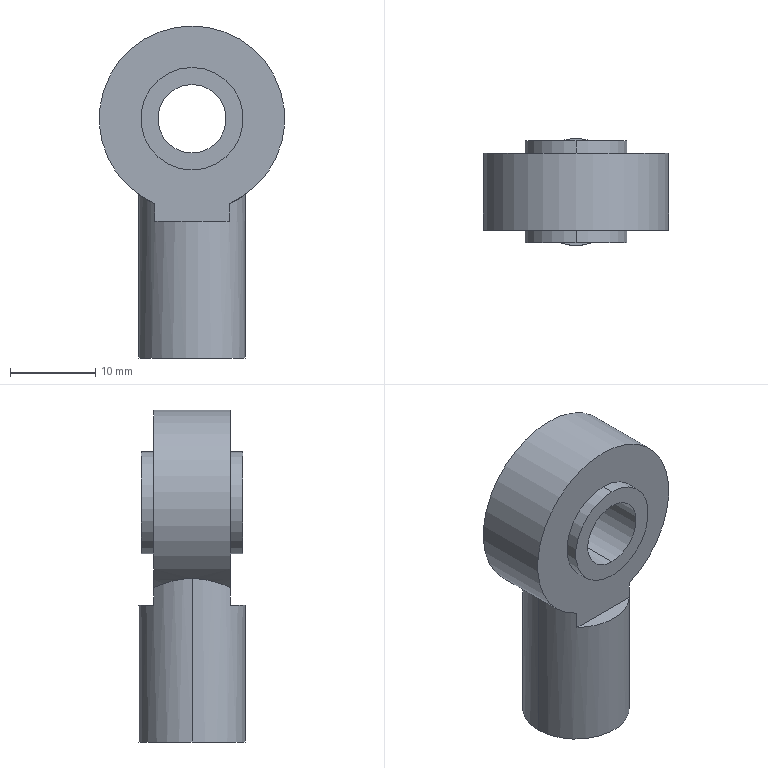Part | SolidWorks | features ICE 4, Extrusion 1, HoleWzd 1 | 1 solid | 20 faces | box 21.7 x 12.5 x 38.85 mm | volume 4732 mm3 | cylinder 11 | plane 7 | cone 2 | commonest cylinder face diameters 12 x4 6.8 x2 8 x2 12.5 x2 21.7 x1
STEP:
#1=CARTESIAN_POINT('',(0.,5.95,24.));
#2=VERTEX_POINT('',#1);
#3=CARTESIAN_POINT('',(0.,5.95,32.));
#4=VERTEX_POINT('',#3);
#5=CARTESIAN_POINT('',(0.,5.95,28.));
#6=DIRECTION('',(0.,1.,0.));
#7=DIRECTION('',(0.,0.,1.));
#8=AXIS2_PLACEMENT_3D('',#5,#6,#7);
#9=CIRCLE('',#8,4.);
#10=EDGE_CURVE('',#2,#4,#9,.T.);
#11=ORIENTED_EDGE('',*,*,#10,.T.);
#12=CARTESIAN_POINT('',(0.,-5.95,32.));
#13=VERTEX_POINT('',#12);
#14=CARTESIAN_POINT('',(0.,6.25,32.));
#15=DIRECTION('',(0.,-1.,0.));
#16=VECTOR('',#15,1000.);
#17=LINE('',#14,#16);
#18=EDGE_CURVE('',#4,#13,#17,.T.);
#19=ORIENTED_EDGE('',*,*,#18,.T.);
#20=CARTESIAN_POINT('',(0.,-5.95,24.));
#21=VERTEX_POINT('',#20);
#22=CARTESIAN_POINT('',(0.,-5.95,28.));
#23=DIRECTION('',(0.,1.,0.));
#24=DIRECTION('',(0.,0.,1.));
#25=AXIS2_PLACEMENT_3D('',#22,#23,#24);
#26=CIRCLE('',#25,4.);
#27=EDGE_CURVE('',#21,#13,#26,.T.);
#28=ORIENTED_EDGE('',*,*,#27,.F.);
#29=CARTESIAN_POINT('',(0.,6.25,24.));
#30=DIRECTION('',(0.,-1.,0.));
#31=VECTOR('',#30,1000.);
#32=LINE('',#29,#31);
#33=EDGE_CURVE('',#2,#21,#32,.T.);
#34=ORIENTED_EDGE('',*,*,#33,.F.);
#35=EDGE_LOOP('',(#11,#19,#28,#34));
#36=FACE_OUTER_BOUND('',#35,.T.);
#37=CARTESIAN_POINT('',(0.,6.25,28.));
#38=DIRECTION('',(0.,-1.,0.));
#39=DIRECTION('',(0.,0.,-1.));
#40=AXIS2_PLACEMENT_3D('',#37,#38,#39);
#41=CYLINDRICAL_SURFACE('',#40,4.);
#42=ADVANCED_FACE('',(#36),#41,.F.);
#43=CARTESIAN_POINT('',(0.,5.95,34.));
#44=VERTEX_POINT('',#43);
#45=CARTESIAN_POINT('',(0.,5.95,22.));
#46=VERTEX_POINT('',#45);
#47=CARTESIAN_POINT('',(0.,5.95,28.));
#48=DIRECTION('',(0.,1.,0.));
#49=DIRECTION('',(0.,0.,1.));
#50=AXIS2_PLACEMENT_3D('',#47,#48,#49);
#51=CIRCLE('',#50,6.);
#52=EDGE_CURVE('',#44,#46,#51,.T.);
#53=ORIENTED_EDGE('',*,*,#52,.F.);
#54=CARTESIAN_POINT('',(0.,4.5,34.));
#55=VERTEX_POINT('',#54);
#56=CARTESIAN_POINT('',(0.,5.95,34.));
#57=DIRECTION('',(0.,-1.,0.));
#58=VECTOR('',#57,1000.);
#59=LINE('',#56,#58);
#60=EDGE_CURVE('',#44,#55,#59,.T.);
#61=ORIENTED_EDGE('',*,*,#60,.T.);
#62=CARTESIAN_POINT('',(0.,4.5,22.));
#63=VERTEX_POINT('',#62);
#64=CARTESIAN_POINT('',(0.,4.5,28.));
#65=DIRECTION('',(0.,-1.,0.));
#66=DIRECTION('',(0.,0.,1.));
#67=AXIS2_PLACEMENT_3D('',#64,#65,#66);
#68=CIRCLE('',#67,6.);
#69=EDGE_CURVE('',#63,#55,#68,.T.);
#70=ORIENTED_EDGE('',*,*,#69,.F.);
#71=CARTESIAN_POINT('',(0.,5.95,22.));
#72=DIRECTION('',(0.,-1.,0.));
#73=VECTOR('',#72,1000.);
#74=LINE('',#71,#73);
#75=EDGE_CURVE('',#46,#63,#74,.T.);
#76=ORIENTED_EDGE('',*,*,#75,.F.);
#77=EDGE_LOOP('',(#53,#61,#70,#76));
#78=FACE_OUTER_BOUND('',#77,.T.);
#79=CARTESIAN_POINT('',(0.,5.95,28.));
#80=DIRECTION('',(0.,-1.,0.));
#81=DIRECTION('',(0.,0.,-1.));
#82=AXIS2_PLACEMENT_3D('',#79,#80,#81);
#83=CYLINDRICAL_SURFACE('',#82,6.);
#84=ADVANCED_FACE('',(#78),#83,.T.);
#85=CARTESIAN_POINT('',(0.,-4.5,22.));
#86=VERTEX_POINT('',#85);
#87=CARTESIAN_POINT('',(0.,-4.5,34.));
#88=VERTEX_POINT('',#87);
#89=CARTESIAN_POINT('',(0.,-4.5,28.));
#90=DIRECTION('',(0.,-1.,0.));
#91=DIRECTION('',(0.,0.,1.));
#92=AXIS2_PLACEMENT_3D('',#89,#90,#91);
#93=CIRCLE('',#92,6.);
#94=EDGE_CURVE('',#86,#88,#93,.T.);
#95=ORIENTED_EDGE('',*,*,#94,.T.);
#96=CARTESIAN_POINT('',(0.,-5.95,34.));
#97=VERTEX_POINT('',#96);
#98=CARTESIAN_POINT('',(0.,5.95,34.));
#99=DIRECTION('',(0.,-1.,0.));
#100=VECTOR('',#99,1000.);
#101=LINE('',#98,#100);
#102=EDGE_CURVE('',#88,#97,#101,.T.);
#103=ORIENTED_EDGE('',*,*,#102,.T.);
#104=CARTESIAN_POINT('',(0.,-5.95,22.));
#105=VERTEX_POINT('',#104);
#106=CARTESIAN_POINT('',(0.,-5.95,28.));
#107=DIRECTION('',(0.,1.,0.));
#108=DIRECTION('',(0.,0.,1.));
#109=AXIS2_PLACEMENT_3D('',#106,#107,#108);
#110=CIRCLE('',#109,6.);
#111=EDGE_CURVE('',#97,#105,#110,.T.);
#112=ORIENTED_EDGE('',*,*,#111,.T.);
#113=CARTESIAN_POINT('',(0.,5.95,22.));
#114=DIRECTION('',(0.,-1.,0.));
#115=VECTOR('',#114,1000.);
#116=LINE('',#113,#115);
#117=EDGE_CURVE('',#86,#105,#116,.T.);
#118=ORIENTED_EDGE('',*,*,#117,.F.);
#119=EDGE_LOOP('',(#95,#103,#112,#118));
#120=FACE_OUTER_BOUND('',#119,.T.);
#121=CARTESIAN_POINT('',(0.,5.95,28.));
#122=DIRECTION('',(0.,-1.,0.));
#123=DIRECTION('',(0.,0.,-1.));
#124=AXIS2_PLACEMENT_3D('',#121,#122,#123);
#125=CYLINDRICAL_SURFACE('',#124,6.);
#126=ADVANCED_FACE('',(#120),#125,.T.);
#127=CARTESIAN_POINT('',(3.4,0.,12.));
#128=VERTEX_POINT('',#127);
#129=CARTESIAN_POINT('',(-3.4,0.,12.));
#130=VERTEX_POINT('',#129);
#131=CARTESIAN_POINT('',(0.,0.,12.));
#132=DIRECTION('',(0.,0.,-1.));
#133=DIRECTION('',(-1.,0.,0.));
#134=AXIS2_PLACEMENT_3D('',#131,#132,#133);
#135=CIRCLE('',#134,3.4);
#136=EDGE_CURVE('',#128,#130,#135,.T.);
#137=ORIENTED_EDGE('',*,*,#136,.F.);
#138=CARTESIAN_POINT('',(3.4,0.,0.));
#139=VERTEX_POINT('',#138);
#140=CARTESIAN_POINT('',(3.4,0.,0.));
#141=DIRECTION('',(0.,0.,-1.));
#142=VECTOR('',#141,1000.);
#143=LINE('',#140,#142);
#144=EDGE_CURVE('',#128,#139,#143,.T.);
#145=ORIENTED_EDGE('',*,*,#144,.T.);
#146=CARTESIAN_POINT('',(-3.4,0.,0.));
#147=VERTEX_POINT('',#146);
#148=CARTESIAN_POINT('',(0.,0.,0.));
#149=DIRECTION('',(0.,0.,-1.));
#150=DIRECTION('',(-1.,0.,0.));
#151=AXIS2_PLACEMENT_3D('',#148,#149,#150);
#152=CIRCLE('',#151,3.4);
#153=EDGE_CURVE('',#139,#147,#152,.T.);
#154=ORIENTED_EDGE('',*,*,#153,.T.);
#155=CARTESIAN_POINT('',(-3.4,0.,0.));
#156=DIRECTION('',(0.,0.,-1.));
#157=VECTOR('',#156,1000.);
#158=LINE('',#155,#157);
#159=EDGE_CURVE('',#130,#147,#158,.T.);
#160=ORIENTED_EDGE('',*,*,#159,.F.);
#161=EDGE_LOOP('',(#137,#145,#154,#160));
#162=FACE_OUTER_BOUND('',#161,.T.);
#163=CARTESIAN_POINT('',(0.,0.,0.));
#164=DIRECTION('',(0.,0.,-1.));
#165=DIRECTION('',(-1.,0.,0.));
#166=AXIS2_PLACEMENT_3D('',#163,#164,#165);
#167=CYLINDRICAL_SURFACE('',#166,3.4);
#168=ADVANCED_FACE('',(#162),#167,.F.);
#169=CARTESIAN_POINT('',(0.,0.,14.043));
#170=VERTEX_POINT('',#169);
#171=CARTESIAN_POINT('',(-3.4,0.,12.));
#172=DIRECTION('',(-0.8572,0.,-0.515));
#173=VECTOR('',#172,1000.);
#174=LINE('',#171,#173);
#175=EDGE_CURVE('',#170,#130,#174,.T.);
#176=ORIENTED_EDGE('',*,*,#175,.F.);
#177=CARTESIAN_POINT('',(3.4,0.,12.));
#178=DIRECTION('',(0.8572,0.,-0.515));
#179=VECTOR('',#178,1000.);
#180=LINE('',#177,#179);
#181=EDGE_CURVE('',#170,#128,#180,.T.);
#182=ORIENTED_EDGE('',*,*,#181,.T.);
#183=ORIENTED_EDGE('',*,*,#136,.T.);
#184=EDGE_LOOP('',(#176,#182,#183));
#185=FACE_OUTER_BOUND('',#184,.T.);
#186=CARTESIAN_POINT('',(0.,0.,12.));
#187=DIRECTION('',(0.,0.,-1.));
#188=DIRECTION('',(-1.,0.,0.));
#189=AXIS2_PLACEMENT_3D('',#186,#187,#188);
#190=CONICAL_SURFACE('',#189,3.4,1.03);
#191=ADVANCED_FACE('',(#185),#190,.F.);
#192=CARTESIAN_POINT('',(6.25,0.,19.131));
#193=VERTEX_POINT('',#192);
#194=CARTESIAN_POINT('',(4.337,4.5,18.055));
#195=VERTEX_POINT('',#194);
#196=CARTESIAN_POINT('',(6.25,0.,19.131));
#197=CARTESIAN_POINT('',(6.25,0.4269,19.131));
#198=CARTESIAN_POINT('',(6.206,0.8535,19.1));
#199=CARTESIAN_POINT('',(6.032,1.693,18.98));
#200=CARTESIAN_POINT('',(5.904,2.094,18.895));
#201=CARTESIAN_POINT('',(5.655,2.669,18.74));
#202=CARTESIAN_POINT('',(5.562,2.857,18.684));
#203=CARTESIAN_POINT('',(5.361,3.22,18.566));
#204=CARTESIAN_POINT('',(5.252,3.394,18.505));
#205=CARTESIAN_POINT('',(4.901,3.9,18.317));
#206=CARTESIAN_POINT('',(4.635,4.213,18.184));
#207=CARTESIAN_POINT('',(4.337,4.5,18.055));
#208=B_SPLINE_CURVE_WITH_KNOTS('',3,(#196,#197,#198,#199,#200,#201,#202,#203,#204,#205,#206,#207),.UNSPECIFIED.,.F.,.F.,(4,2,2,2,2,4),(0.005141,0.006422,0.007703,0.008344,0.008985,0.01027),.UNSPECIFIED.);
#209=EDGE_CURVE('',#193,#195,#208,.T.);
#210=ORIENTED_EDGE('',*,*,#209,.F.);
#211=CARTESIAN_POINT('',(6.25,0.,0.));
#212=VERTEX_POINT('',#211);
#213=CARTESIAN_POINT('',(6.25,0.,28.));
#214=DIRECTION('',(0.,0.,-1.));
#215=VECTOR('',#214,1000.);
#216=LINE('',#213,#215);
#217=EDGE_CURVE('',#193,#212,#216,.T.);
#218=ORIENTED_EDGE('',*,*,#217,.T.);
#219=CARTESIAN_POINT('',(-6.25,0.,0.));
#220=VERTEX_POINT('',#219);
#221=CARTESIAN_POINT('',(0.,0.,0.));
#222=DIRECTION('',(0.,0.,1.));
#223=DIRECTION('',(1.,0.,0.));
#224=AXIS2_PLACEMENT_3D('',#221,#222,#223);
#225=CIRCLE('',#224,6.25);
#226=EDGE_CURVE('',#212,#220,#225,.T.);
#227=ORIENTED_EDGE('',*,*,#226,.T.);
#228=CARTESIAN_POINT('',(-6.25,0.,19.131));
#229=VERTEX_POINT('',#228);
#230=CARTESIAN_POINT('',(-6.25,0.,28.));
#231=DIRECTION('',(0.,0.,-1.));
#232=VECTOR('',#231,1000.);
#233=LINE('',#230,#232);
#234=EDGE_CURVE('',#229,#220,#233,.T.);
#235=ORIENTED_EDGE('',*,*,#234,.F.);
#236=CARTESIAN_POINT('',(-4.337,4.5,18.055));
#237=VERTEX_POINT('',#236);
#238=CARTESIAN_POINT('',(-4.337,4.5,18.055));
#239=CARTESIAN_POINT('',(-4.635,4.213,18.185));
#240=CARTESIAN_POINT('',(-4.9,3.901,18.316));
#241=CARTESIAN_POINT('',(-5.251,3.396,18.504));
#242=CARTESIAN_POINT('',(-5.36,3.222,18.566));
#243=CARTESIAN_POINT('',(-5.562,2.859,18.683));
#244=CARTESIAN_POINT('',(-5.655,2.67,18.74));
#245=CARTESIAN_POINT('',(-5.903,2.095,18.894));
#246=CARTESIAN_POINT('',(-6.03,1.696,18.98));
#247=CARTESIAN_POINT('',(-6.161,1.073,19.069));
#248=CARTESIAN_POINT('',(-6.194,0.8594,19.092));
#249=CARTESIAN_POINT('',(-6.239,0.4288,19.123));
#250=CARTESIAN_POINT('',(-6.25,0.2141,19.131));
#251=CARTESIAN_POINT('',(-6.25,0.,19.131));
#252=B_SPLINE_CURVE_WITH_KNOTS('',3,(#238,#239,#240,#241,#242,#243,#244,#245,#246,#247,#248,#249,#250,#251),.UNSPECIFIED.,.F.,.F.,(4,2,2,2,2,2,4),(0.,0.001285,0.001928,0.00257,0.003856,0.004498,0.005141),.UNSPECIFIED.);
#253=EDGE_CURVE('',#237,#229,#252,.T.);
#254=ORIENTED_EDGE('',*,*,#253,.F.);
#255=CARTESIAN_POINT('',(-4.337,4.5,16.));
#256=VERTEX_POINT('',#255);
#257=CARTESIAN_POINT('',(-4.337,4.5,16.));
#258=DIRECTION('',(0.,0.,1.));
#259=VECTOR('',#258,1000.);
#260=LINE('',#257,#259);
#261=EDGE_CURVE('',#256,#237,#260,.T.);
#262=ORIENTED_EDGE('',*,*,#261,.F.);
#263=CARTESIAN_POINT('',(4.337,4.5,16.));
#264=VERTEX_POINT('',#263);
#265=CARTESIAN_POINT('',(0.,0.,16.));
#266=DIRECTION('',(0.,0.,1.));
#267=DIRECTION('',(1.,0.,0.));
#268=AXIS2_PLACEMENT_3D('',#265,#266,#267);
#269=CIRCLE('',#268,6.25);
#270=EDGE_CURVE('',#264,#256,#269,.T.);
#271=ORIENTED_EDGE('',*,*,#270,.F.);
#272=CARTESIAN_POINT('',(4.337,4.5,16.));
#273=DIRECTION('',(0.,0.,1.));
#274=VECTOR('',#273,1000.);
#275=LINE('',#272,#274);
#276=EDGE_CURVE('',#264,#195,#275,.T.);
#277=ORIENTED_EDGE('',*,*,#276,.T.);
#278=EDGE_LOOP('',(#210,#218,#227,#235,#254,#262,#271,#277));
#279=FACE_OUTER_BOUND('',#278,.T.);
#280=CARTESIAN_POINT('',(0.,0.,28.));
#281=DIRECTION('',(0.,0.,-1.));
#282=DIRECTION('',(-1.,0.,0.));
#283=AXIS2_PLACEMENT_3D('',#280,#281,#282);
#284=CYLINDRICAL_SURFACE('',#283,6.25);
#285=ADVANCED_FACE('',(#279),#284,.T.);
#286=CARTESIAN_POINT('',(0.,4.5,28.));
#287=DIRECTION('',(0.,1.,0.));
#288=DIRECTION('',(0.,0.,1.));
#289=AXIS2_PLACEMENT_3D('',#286,#287,#288);
#290=CIRCLE('',#289,10.85);
#291=EDGE_CURVE('',#237,#195,#290,.T.);
#292=ORIENTED_EDGE('',*,*,#291,.T.);
#293=ORIENTED_EDGE('',*,*,#276,.F.);
#294=CARTESIAN_POINT('',(-4.337,4.5,16.));
#295=DIRECTION('',(1.,0.,0.));
#296=VECTOR('',#295,1000.);
#297=LINE('',#294,#296);
#298=EDGE_CURVE('',#256,#264,#297,.T.);
#299=ORIENTED_EDGE('',*,*,#298,.F.);
#300=ORIENTED_EDGE('',*,*,#261,.T.);
#301=EDGE_LOOP('',(#292,#293,#299,#300));
#302=FACE_OUTER_BOUND('',#301,.T.);
#303=ORIENTED_EDGE('',*,*,#69,.T.);
#304=CARTESIAN_POINT('',(0.,4.5,28.));
#305=DIRECTION('',(0.,-1.,0.));
#306=DIRECTION('',(0.,0.,1.));
#307=AXIS2_PLACEMENT_3D('',#304,#305,#306);
#308=CIRCLE('',#307,6.);
#309=EDGE_CURVE('',#55,#63,#308,.T.);
#310=ORIENTED_EDGE('',*,*,#309,.T.);
#311=EDGE_LOOP('',(#303,#310));
#312=FACE_BOUND('',#311,.T.);
#313=CARTESIAN_POINT('',(0.,4.5,28.));
#314=DIRECTION('',(0.,1.,0.));
#315=DIRECTION('',(0.,0.,1.));
#316=AXIS2_PLACEMENT_3D('',#313,#314,#315);
#317=PLANE('',#316);
#318=ADVANCED_FACE('',(#302,#312),#317,.T.);
#319=CARTESIAN_POINT('',(4.337,-4.5,16.));
#320=VERTEX_POINT('',#319);
#321=CARTESIAN_POINT('',(4.337,-4.5,18.055));
#322=VERTEX_POINT('',#321);
#323=CARTESIAN_POINT('',(4.337,-4.5,16.));
#324=DIRECTION('',(0.,0.,1.));
#325=VECTOR('',#324,1000.);
#326=LINE('',#323,#325);
#327=EDGE_CURVE('',#320,#322,#326,.T.);
#328=ORIENTED_EDGE('',*,*,#327,.T.);
#329=CARTESIAN_POINT('',(-4.337,-4.5,18.055));
#330=VERTEX_POINT('',#329);
#331=CARTESIAN_POINT('',(0.,-4.5,28.));
#332=DIRECTION('',(0.,1.,0.));
#333=DIRECTION('',(0.,0.,1.));
#334=AXIS2_PLACEMENT_3D('',#331,#332,#333);
#335=CIRCLE('',#334,10.85);
#336=EDGE_CURVE('',#330,#322,#335,.T.);
#337=ORIENTED_EDGE('',*,*,#336,.F.);
#338=CARTESIAN_POINT('',(-4.337,-4.5,16.));
#339=VERTEX_POINT('',#338);
#340=CARTESIAN_POINT('',(-4.337,-4.5,16.));
#341=DIRECTION('',(0.,0.,1.));
#342=VECTOR('',#341,1000.);
#343=LINE('',#340,#342);
#344=EDGE_CURVE('',#339,#330,#343,.T.);
#345=ORIENTED_EDGE('',*,*,#344,.F.);
#346=CARTESIAN_POINT('',(4.337,-4.5,16.));
#347=DIRECTION('',(-1.,0.,0.));
#348=VECTOR('',#347,1000.);
#349=LINE('',#346,#348);
#350=EDGE_CURVE('',#320,#339,#349,.T.);
#351=ORIENTED_EDGE('',*,*,#350,.F.);
#352=EDGE_LOOP('',(#328,#337,#345,#351));
#353=FACE_OUTER_BOUND('',#352,.T.);
#354=ORIENTED_EDGE('',*,*,#94,.F.);
#355=CARTESIAN_POINT('',(0.,-4.5,28.));
#356=DIRECTION('',(0.,-1.,0.));
#357=DIRECTION('',(0.,0.,1.));
#358=AXIS2_PLACEMENT_3D('',#355,#356,#357);
#359=CIRCLE('',#358,6.);
#360=EDGE_CURVE('',#88,#86,#359,.T.);
#361=ORIENTED_EDGE('',*,*,#360,.F.);
#362=EDGE_LOOP('',(#354,#361));
#363=FACE_BOUND('',#362,.T.);
#364=CARTESIAN_POINT('',(0.,-4.5,28.));
#365=DIRECTION('',(0.,1.,0.));
#366=DIRECTION('',(0.,0.,1.));
#367=AXIS2_PLACEMENT_3D('',#364,#365,#366);
#368=PLANE('',#367);
#369=ADVANCED_FACE('',(#353,#363),#368,.F.);
#370=ORIENTED_EDGE('',*,*,#217,.F.);
#371=CARTESIAN_POINT('',(4.337,-4.5,18.055));
#372=CARTESIAN_POINT('',(4.635,-4.213,18.185));
#373=CARTESIAN_POINT('',(4.9,-3.901,18.316));
#374=CARTESIAN_POINT('',(5.251,-3.396,18.504));
#375=CARTESIAN_POINT('',(5.36,-3.222,18.566));
#376=CARTESIAN_POINT('',(5.562,-2.859,18.683));
#377=CARTESIAN_POINT('',(5.655,-2.67,18.74));
#378=CARTESIAN_POINT('',(5.903,-2.095,18.894));
#379=CARTESIAN_POINT('',(6.03,-1.696,18.98));
#380=CARTESIAN_POINT('',(6.161,-1.073,19.069));
#381=CARTESIAN_POINT('',(6.194,-0.8594,19.092));
#382=CARTESIAN_POINT('',(6.239,-0.4288,19.123));
#383=CARTESIAN_POINT('',(6.25,-0.2141,19.131));
#384=CARTESIAN_POINT('',(6.25,0.,19.131));
#385=B_SPLINE_CURVE_WITH_KNOTS('',3,(#371,#372,#373,#374,#375,#376,#377,#378,#379,#380,#381,#382,#383,#384),.UNSPECIFIED.,.F.,.F.,(4,2,2,2,2,2,4),(0.,0.001285,0.001928,0.00257,0.003856,0.004498,0.005141),.UNSPECIFIED.);
#386=EDGE_CURVE('',#322,#193,#385,.T.);
#387=ORIENTED_EDGE('',*,*,#386,.F.);
#388=ORIENTED_EDGE('',*,*,#327,.F.);
#389=CARTESIAN_POINT('',(0.,0.,16.));
#390=DIRECTION('',(0.,0.,1.));
#391=DIRECTION('',(1.,0.,0.));
#392=AXIS2_PLACEMENT_3D('',#389,#390,#391);
#393=CIRCLE('',#392,6.25);
#394=EDGE_CURVE('',#339,#320,#393,.T.);
#395=ORIENTED_EDGE('',*,*,#394,.F.);
#396=ORIENTED_EDGE('',*,*,#344,.T.);
#397=CARTESIAN_POINT('',(-6.25,0.,19.131));
#398=CARTESIAN_POINT('',(-6.25,-0.4269,19.131));
#399=CARTESIAN_POINT('',(-6.206,-0.8535,19.1));
#400=CARTESIAN_POINT('',(-6.032,-1.693,18.98));
#401=CARTESIAN_POINT('',(-5.904,-2.094,18.895));
#402=CARTESIAN_POINT('',(-5.655,-2.669,18.74));
#403=CARTESIAN_POINT('',(-5.562,-2.857,18.684));
#404=CARTESIAN_POINT('',(-5.361,-3.22,18.566));
#405=CARTESIAN_POINT('',(-5.252,-3.394,18.505));
#406=CARTESIAN_POINT('',(-4.901,-3.9,18.317));
#407=CARTESIAN_POINT('',(-4.635,-4.213,18.184));
#408=CARTESIAN_POINT('',(-4.337,-4.5,18.055));
#409=B_SPLINE_CURVE_WITH_KNOTS('',3,(#397,#398,#399,#400,#401,#402,#403,#404,#405,#406,#407,#408),.UNSPECIFIED.,.F.,.F.,(4,2,2,2,2,4),(0.005141,0.006422,0.007703,0.008344,0.008985,0.01027),.UNSPECIFIED.);
#410=EDGE_CURVE('',#229,#330,#409,.T.);
#411=ORIENTED_EDGE('',*,*,#410,.F.);
#412=ORIENTED_EDGE('',*,*,#234,.T.);
#413=CARTESIAN_POINT('',(0.,0.,0.));
#414=DIRECTION('',(0.,0.,1.));
#415=DIRECTION('',(1.,0.,0.));
#416=AXIS2_PLACEMENT_3D('',#413,#414,#415);
#417=CIRCLE('',#416,6.25);
#418=EDGE_CURVE('',#220,#212,#417,.T.);
#419=ORIENTED_EDGE('',*,*,#418,.T.);
#420=EDGE_LOOP('',(#370,#387,#388,#395,#396,#411,#412,#419));
#421=FACE_OUTER_BOUND('',#420,.T.);
#422=CARTESIAN_POINT('',(0.,0.,28.));
#423=DIRECTION('',(0.,0.,-1.));
#424=DIRECTION('',(-1.,0.,0.));
#425=AXIS2_PLACEMENT_3D('',#422,#423,#424);
#426=CYLINDRICAL_SURFACE('',#425,6.25);
#427=ADVANCED_FACE('',(#421),#426,.T.);
#428=CARTESIAN_POINT('',(0.,0.,0.));
#429=DIRECTION('',(0.,0.,-1.));
#430=DIRECTION('',(-1.,0.,0.));
#431=AXIS2_PLACEMENT_3D('',#428,#429,#430);
#432=CIRCLE('',#431,3.4);
#433=EDGE_CURVE('',#147,#139,#432,.T.);
#434=ORIENTED_EDGE('',*,*,#433,.F.);
#435=ORIENTED_EDGE('',*,*,#153,.F.);
#436=EDGE_LOOP('',(#434,#435));
#437=FACE_BOUND('',#436,.T.);
#438=ORIENTED_EDGE('',*,*,#418,.F.);
#439=ORIENTED_EDGE('',*,*,#226,.F.);
#440=EDGE_LOOP('',(#438,#439));
#441=FACE_OUTER_BOUND('',#440,.T.);
#442=CARTESIAN_POINT('',(0.,0.,0.));
#443=DIRECTION('',(0.,0.,1.));
#444=DIRECTION('',(1.,0.,0.));
#445=AXIS2_PLACEMENT_3D('',#442,#443,#444);
#446=PLANE('',#445);
#447=ADVANCED_FACE('',(#437,#441),#446,.F.);
#448=ORIENTED_EDGE('',*,*,#291,.F.);
#449=ORIENTED_EDGE('',*,*,#253,.T.);
#450=ORIENTED_EDGE('',*,*,#410,.T.);
#451=ORIENTED_EDGE('',*,*,#336,.T.);
#452=ORIENTED_EDGE('',*,*,#386,.T.);
#453=ORIENTED_EDGE('',*,*,#209,.T.);
#454=EDGE_LOOP('',(#448,#449,#450,#451,#452,#453));
#455=FACE_OUTER_BOUND('',#454,.T.);
#456=CARTESIAN_POINT('',(0.,4.5,28.));
#457=DIRECTION('',(0.,-1.,0.));
#458=DIRECTION('',(0.,0.,-1.));
#459=AXIS2_PLACEMENT_3D('',#456,#457,#458);
#460=CYLINDRICAL_SURFACE('',#459,10.85);
#461=ADVANCED_FACE('',(#455),#460,.T.);
#462=ORIENTED_EDGE('',*,*,#270,.T.);
#463=ORIENTED_EDGE('',*,*,#298,.T.);
#464=EDGE_LOOP('',(#462,#463));
#465=FACE_OUTER_BOUND('',#464,.T.);
#466=CARTESIAN_POINT('',(0.,0.,16.));
#467=DIRECTION('',(0.,0.,1.));
#468=DIRECTION('',(1.,0.,0.));
#469=AXIS2_PLACEMENT_3D('',#466,#467,#468);
#470=PLANE('',#469);
#471=ADVANCED_FACE('',(#465),#470,.T.);
#472=ORIENTED_EDGE('',*,*,#394,.T.);
#473=ORIENTED_EDGE('',*,*,#350,.T.);
#474=EDGE_LOOP('',(#472,#473));
#475=FACE_OUTER_BOUND('',#474,.T.);
#476=CARTESIAN_POINT('',(0.,0.,16.));
#477=DIRECTION('',(0.,0.,1.));
#478=DIRECTION('',(1.,0.,0.));
#479=AXIS2_PLACEMENT_3D('',#476,#477,#478);
#480=PLANE('',#479);
#481=ADVANCED_FACE('',(#475),#480,.T.);
#482=ORIENTED_EDGE('',*,*,#181,.F.);
#483=ORIENTED_EDGE('',*,*,#175,.T.);
#484=CARTESIAN_POINT('',(0.,0.,12.));
#485=DIRECTION('',(0.,0.,-1.));
#486=DIRECTION('',(-1.,0.,0.));
#487=AXIS2_PLACEMENT_3D('',#484,#485,#486);
#488=CIRCLE('',#487,3.4);
#489=EDGE_CURVE('',#130,#128,#488,.T.);
#490=ORIENTED_EDGE('',*,*,#489,.T.);
#491=EDGE_LOOP('',(#482,#483,#490));
#492=FACE_OUTER_BOUND('',#491,.T.);
#493=CARTESIAN_POINT('',(0.,0.,12.));
#494=DIRECTION('',(0.,0.,-1.));
#495=DIRECTION('',(-1.,0.,0.));
#496=AXIS2_PLACEMENT_3D('',#493,#494,#495);
#497=CONICAL_SURFACE('',#496,3.4,1.03);
#498=ADVANCED_FACE('',(#492),#497,.F.);
#499=ORIENTED_EDGE('',*,*,#144,.F.);
#500=ORIENTED_EDGE('',*,*,#489,.F.);
#501=ORIENTED_EDGE('',*,*,#159,.T.);
#502=ORIENTED_EDGE('',*,*,#433,.T.);
#503=EDGE_LOOP('',(#499,#500,#501,#502));
#504=FACE_OUTER_BOUND('',#503,.T.);
#505=CARTESIAN_POINT('',(0.,0.,0.));
#506=DIRECTION('',(0.,0.,-1.));
#507=DIRECTION('',(-1.,0.,0.));
#508=AXIS2_PLACEMENT_3D('',#505,#506,#507);
#509=CYLINDRICAL_SURFACE('',#508,3.4);
#510=ADVANCED_FACE('',(#504),#509,.F.);
#511=ORIENTED_EDGE('',*,*,#102,.F.);
#512=ORIENTED_EDGE('',*,*,#360,.T.);
#513=ORIENTED_EDGE('',*,*,#117,.T.);
#514=CARTESIAN_POINT('',(0.,-5.95,28.));
#515=DIRECTION('',(0.,1.,0.));
#516=DIRECTION('',(0.,0.,1.));
#517=AXIS2_PLACEMENT_3D('',#514,#515,#516);
#518=CIRCLE('',#517,6.);
#519=EDGE_CURVE('',#105,#97,#518,.T.);
#520=ORIENTED_EDGE('',*,*,#519,.T.);
#521=EDGE_LOOP('',(#511,#512,#513,#520));
#522=FACE_OUTER_BOUND('',#521,.T.);
#523=CARTESIAN_POINT('',(0.,5.95,28.));
#524=DIRECTION('',(0.,-1.,0.));
#525=DIRECTION('',(0.,0.,-1.));
#526=AXIS2_PLACEMENT_3D('',#523,#524,#525);
#527=CYLINDRICAL_SURFACE('',#526,6.);
#528=ADVANCED_FACE('',(#522),#527,.T.);
#529=ORIENTED_EDGE('',*,*,#519,.F.);
#530=ORIENTED_EDGE('',*,*,#111,.F.);
#531=EDGE_LOOP('',(#529,#530));
#532=FACE_OUTER_BOUND('',#531,.T.);
#533=ORIENTED_EDGE('',*,*,#27,.T.);
#534=CARTESIAN_POINT('',(0.,-5.95,28.));
#535=DIRECTION('',(0.,1.,0.));
#536=DIRECTION('',(0.,0.,1.));
#537=AXIS2_PLACEMENT_3D('',#534,#535,#536);
#538=CIRCLE('',#537,4.);
#539=EDGE_CURVE('',#13,#21,#538,.T.);
#540=ORIENTED_EDGE('',*,*,#539,.T.);
#541=EDGE_LOOP('',(#533,#540));
#542=FACE_BOUND('',#541,.T.);
#543=CARTESIAN_POINT('',(0.,-5.95,28.));
#544=DIRECTION('',(0.,1.,0.));
#545=DIRECTION('',(0.,0.,1.));
#546=AXIS2_PLACEMENT_3D('',#543,#544,#545);
#547=PLANE('',#546);
#548=ADVANCED_FACE('',(#532,#542),#547,.F.);
#549=CARTESIAN_POINT('',(0.,5.95,28.));
#550=DIRECTION('',(0.,1.,0.));
#551=DIRECTION('',(0.,0.,1.));
#552=AXIS2_PLACEMENT_3D('',#549,#550,#551);
#553=CIRCLE('',#552,6.);
#554=EDGE_CURVE('',#46,#44,#553,.T.);
#555=ORIENTED_EDGE('',*,*,#554,.T.);
#556=ORIENTED_EDGE('',*,*,#52,.T.);
#557=EDGE_LOOP('',(#555,#556));
#558=FACE_OUTER_BOUND('',#557,.T.);
#559=ORIENTED_EDGE('',*,*,#10,.F.);
#560=CARTESIAN_POINT('',(0.,5.95,28.));
#561=DIRECTION('',(0.,1.,0.));
#562=DIRECTION('',(0.,0.,1.));
#563=AXIS2_PLACEMENT_3D('',#560,#561,#562);
#564=CIRCLE('',#563,4.);
#565=EDGE_CURVE('',#4,#2,#564,.T.);
#566=ORIENTED_EDGE('',*,*,#565,.F.);
#567=EDGE_LOOP('',(#559,#566));
#568=FACE_BOUND('',#567,.T.);
#569=CARTESIAN_POINT('',(0.,5.95,28.));
#570=DIRECTION('',(0.,1.,0.));
#571=DIRECTION('',(0.,0.,1.));
#572=AXIS2_PLACEMENT_3D('',#569,#570,#571);
#573=PLANE('',#572);
#574=ADVANCED_FACE('',(#558,#568),#573,.T.);
#575=ORIENTED_EDGE('',*,*,#60,.F.);
#576=ORIENTED_EDGE('',*,*,#554,.F.);
#577=ORIENTED_EDGE('',*,*,#75,.T.);
#578=ORIENTED_EDGE('',*,*,#309,.F.);
#579=EDGE_LOOP('',(#575,#576,#577,#578));
#580=FACE_OUTER_BOUND('',#579,.T.);
#581=CARTESIAN_POINT('',(0.,5.95,28.));
#582=DIRECTION('',(0.,-1.,0.));
#583=DIRECTION('',(0.,0.,-1.));
#584=AXIS2_PLACEMENT_3D('',#581,#582,#583);
#585=CYLINDRICAL_SURFACE('',#584,6.);
#586=ADVANCED_FACE('',(#580),#585,.T.);
#587=ORIENTED_EDGE('',*,*,#18,.F.);
#588=ORIENTED_EDGE('',*,*,#565,.T.);
#589=ORIENTED_EDGE('',*,*,#33,.T.);
#590=ORIENTED_EDGE('',*,*,#539,.F.);
#591=EDGE_LOOP('',(#587,#588,#589,#590));
#592=FACE_OUTER_BOUND('',#591,.T.);
#593=CARTESIAN_POINT('',(0.,6.25,28.));
#594=DIRECTION('',(0.,-1.,0.));
#595=DIRECTION('',(0.,0.,-1.));
#596=AXIS2_PLACEMENT_3D('',#593,#594,#595);
#597=CYLINDRICAL_SURFACE('',#596,4.);
#598=ADVANCED_FACE('',(#592),#597,.F.);
#599=CLOSED_SHELL('',(#42,#84,#126,#168,#191,#285,#318,#369,#427,#447,#461,#471,#481,#498,#510,#528,#548,#574,#586,#598));
#600=MANIFOLD_SOLID_BREP('',#599);
#601=CARTESIAN_POINT('',(0.,0.,0.));
#602=DIRECTION('',(0.,0.,1.));
#603=DIRECTION('',(1.,0.,0.));
#604=AXIS2_PLACEMENT_3D('',#601,#602,#603);
#605=(LENGTH_UNIT()NAMED_UNIT(*)SI_UNIT(.MILLI.,.METRE.));
#606=UNCERTAINTY_MEASURE_WITH_UNIT(LENGTH_MEASURE(0.00001),#605,'','');
#607=(NAMED_UNIT(*)PLANE_ANGLE_UNIT()SI_UNIT($,.RADIAN.));
#608=(NAMED_UNIT(*)SI_UNIT($,.STERADIAN.)SOLID_ANGLE_UNIT());
#609=(GEOMETRIC_REPRESENTATION_CONTEXT(3)GLOBAL_UNCERTAINTY_ASSIGNED_CONTEXT((#606))GLOBAL_UNIT_ASSIGNED_CONTEXT((#605,#607,#608))REPRESENTATION_CONTEXT('',''));
#610=ADVANCED_BREP_SHAPE_REPRESENTATION('',(#600,#604),#609);